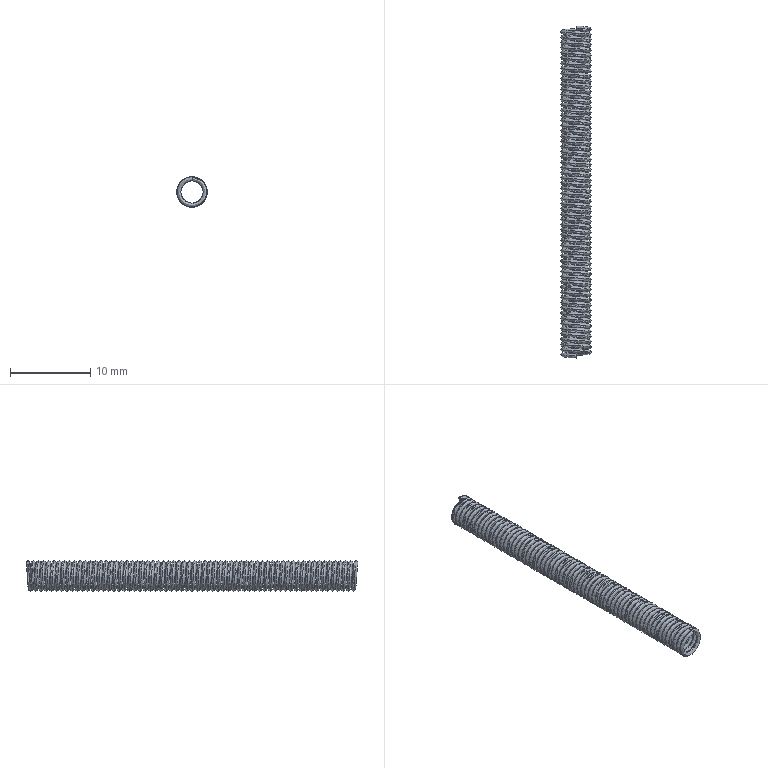Part | SolidWorks | features Helix 1, Sweep 1 | 1 solid | 4 faces | box 3.8 x 41.45 x 3.8 mm | volume 132.538 mm3 | spline 2 | plane 2